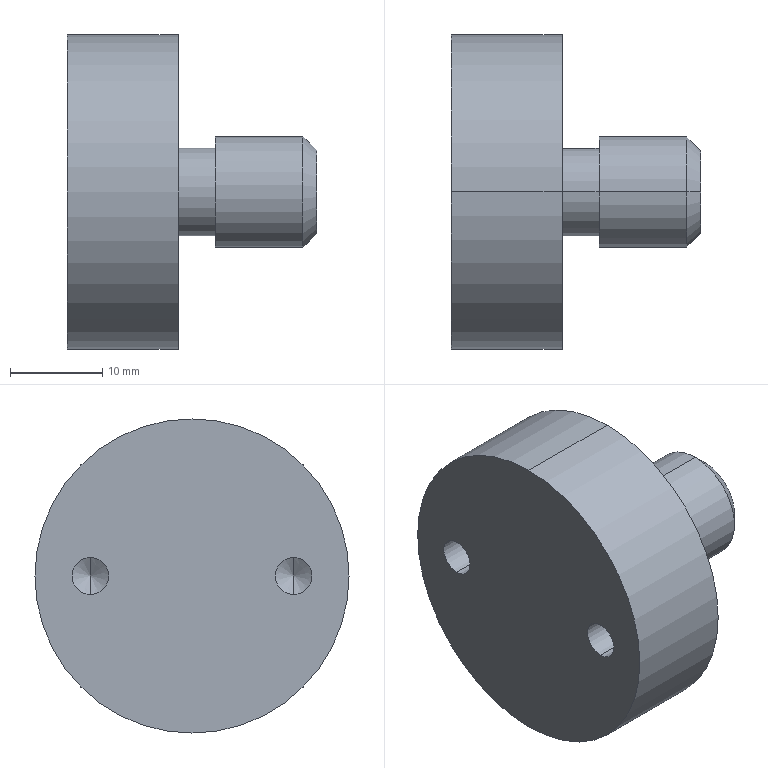Part | SolidWorks | features Chamfer 1, MirrorPattern 1, RevCut 1, Revolution 1 | 1 solid | 20 faces | box 27 x 34 x 34 mm | volume 12223 mm3 | cylinder 10 | cone 6 | plane 4 | commonest cylinder face diameters 4 x4 9.5 x2 12 x2 34 x2
STEP:
#1=CARTESIAN_POINT('',(6.,-11.,2.));
#2=VERTEX_POINT('',#1);
#3=CARTESIAN_POINT('',(6.,-11.,-2.));
#4=VERTEX_POINT('',#3);
#5=CARTESIAN_POINT('',(6.,-11.,0.));
#6=DIRECTION('',(1.,0.,0.));
#7=DIRECTION('',(0.,0.,1.));
#8=AXIS2_PLACEMENT_3D('',#5,#6,#7);
#9=CIRCLE('',#8,2.);
#10=EDGE_CURVE('',#2,#4,#9,.T.);
#11=ORIENTED_EDGE('',*,*,#10,.T.);
#12=CARTESIAN_POINT('',(0.,-11.,-2.));
#13=VERTEX_POINT('',#12);
#14=CARTESIAN_POINT('',(-2.467,-11.,-2.));
#15=DIRECTION('',(-1.,0.,0.));
#16=VECTOR('',#15,1000.);
#17=LINE('',#14,#16);
#18=EDGE_CURVE('',#4,#13,#17,.T.);
#19=ORIENTED_EDGE('',*,*,#18,.T.);
#20=CARTESIAN_POINT('',(0.,-11.,2.));
#21=VERTEX_POINT('',#20);
#22=CARTESIAN_POINT('',(0.,-11.,0.));
#23=DIRECTION('',(1.,0.,0.));
#24=DIRECTION('',(0.,0.,1.));
#25=AXIS2_PLACEMENT_3D('',#22,#23,#24);
#26=CIRCLE('',#25,2.);
#27=EDGE_CURVE('',#21,#13,#26,.T.);
#28=ORIENTED_EDGE('',*,*,#27,.F.);
#29=CARTESIAN_POINT('',(-2.467,-11.,2.));
#30=DIRECTION('',(-1.,0.,0.));
#31=VECTOR('',#30,1000.);
#32=LINE('',#29,#31);
#33=EDGE_CURVE('',#2,#21,#32,.T.);
#34=ORIENTED_EDGE('',*,*,#33,.F.);
#35=EDGE_LOOP('',(#11,#19,#28,#34));
#36=FACE_OUTER_BOUND('',#35,.T.);
#37=CARTESIAN_POINT('',(-2.467,-11.,0.));
#38=DIRECTION('',(-1.,0.,0.));
#39=DIRECTION('',(0.,0.,1.));
#40=AXIS2_PLACEMENT_3D('',#37,#38,#39);
#41=CYLINDRICAL_SURFACE('',#40,2.);
#42=ADVANCED_FACE('',(#36),#41,.F.);
#43=CARTESIAN_POINT('',(7.155,-11.,0.));
#44=VERTEX_POINT('',#43);
#45=CARTESIAN_POINT('',(7.155,-11.,0.));
#46=DIRECTION('',(-0.5,0.,0.866));
#47=VECTOR('',#46,1000.);
#48=LINE('',#45,#47);
#49=EDGE_CURVE('',#44,#2,#48,.T.);
#50=ORIENTED_EDGE('',*,*,#49,.F.);
#51=CARTESIAN_POINT('',(7.155,-11.,0.));
#52=DIRECTION('',(-0.5,0.,-0.866));
#53=VECTOR('',#52,1000.);
#54=LINE('',#51,#53);
#55=EDGE_CURVE('',#44,#4,#54,.T.);
#56=ORIENTED_EDGE('',*,*,#55,.T.);
#57=ORIENTED_EDGE('',*,*,#10,.F.);
#58=EDGE_LOOP('',(#50,#56,#57));
#59=FACE_OUTER_BOUND('',#58,.T.);
#60=CARTESIAN_POINT('',(-992.845,-11.,0.));
#61=DIRECTION('',(-1.,0.,0.));
#62=DIRECTION('',(0.,0.,1.));
#63=AXIS2_PLACEMENT_3D('',#60,#61,#62);
#64=CONICAL_SURFACE('',#63,1732.051,1.047);
#65=ADVANCED_FACE('',(#59),#64,.F.);
#66=CARTESIAN_POINT('',(6.,11.,-2.));
#67=VERTEX_POINT('',#66);
#68=CARTESIAN_POINT('',(6.,11.,2.));
#69=VERTEX_POINT('',#68);
#70=CARTESIAN_POINT('',(6.,11.,0.));
#71=DIRECTION('',(-1.,0.,0.));
#72=DIRECTION('',(0.,0.,1.));
#73=AXIS2_PLACEMENT_3D('',#70,#71,#72);
#74=CIRCLE('',#73,2.);
#75=EDGE_CURVE('',#67,#69,#74,.T.);
#76=ORIENTED_EDGE('',*,*,#75,.F.);
#77=CARTESIAN_POINT('',(0.,11.,-2.));
#78=VERTEX_POINT('',#77);
#79=CARTESIAN_POINT('',(-2.467,11.,-2.));
#80=DIRECTION('',(-1.,0.,0.));
#81=VECTOR('',#80,1000.);
#82=LINE('',#79,#81);
#83=EDGE_CURVE('',#67,#78,#82,.T.);
#84=ORIENTED_EDGE('',*,*,#83,.T.);
#85=CARTESIAN_POINT('',(0.,11.,2.));
#86=VERTEX_POINT('',#85);
#87=CARTESIAN_POINT('',(0.,11.,0.));
#88=DIRECTION('',(-1.,0.,0.));
#89=DIRECTION('',(0.,0.,1.));
#90=AXIS2_PLACEMENT_3D('',#87,#88,#89);
#91=CIRCLE('',#90,2.);
#92=EDGE_CURVE('',#78,#86,#91,.T.);
#93=ORIENTED_EDGE('',*,*,#92,.T.);
#94=CARTESIAN_POINT('',(-2.467,11.,2.));
#95=DIRECTION('',(-1.,0.,0.));
#96=VECTOR('',#95,1000.);
#97=LINE('',#94,#96);
#98=EDGE_CURVE('',#69,#86,#97,.T.);
#99=ORIENTED_EDGE('',*,*,#98,.F.);
#100=EDGE_LOOP('',(#76,#84,#93,#99));
#101=FACE_OUTER_BOUND('',#100,.T.);
#102=CARTESIAN_POINT('',(-2.467,11.,0.));
#103=DIRECTION('',(-1.,0.,0.));
#104=DIRECTION('',(0.,0.,1.));
#105=AXIS2_PLACEMENT_3D('',#102,#103,#104);
#106=CYLINDRICAL_SURFACE('',#105,2.);
#107=ADVANCED_FACE('',(#101),#106,.F.);
#108=CARTESIAN_POINT('',(7.155,11.,0.));
#109=VERTEX_POINT('',#108);
#110=CARTESIAN_POINT('',(7.155,11.,0.));
#111=DIRECTION('',(-0.5,0.,0.866));
#112=VECTOR('',#111,1000.);
#113=LINE('',#110,#112);
#114=EDGE_CURVE('',#109,#69,#113,.T.);
#115=ORIENTED_EDGE('',*,*,#114,.F.);
#116=CARTESIAN_POINT('',(7.155,11.,0.));
#117=DIRECTION('',(-0.5,0.,-0.866));
#118=VECTOR('',#117,1000.);
#119=LINE('',#116,#118);
#120=EDGE_CURVE('',#109,#67,#119,.T.);
#121=ORIENTED_EDGE('',*,*,#120,.T.);
#122=ORIENTED_EDGE('',*,*,#75,.T.);
#123=EDGE_LOOP('',(#115,#121,#122));
#124=FACE_OUTER_BOUND('',#123,.T.);
#125=CARTESIAN_POINT('',(-992.845,11.,0.));
#126=DIRECTION('',(-1.,0.,0.));
#127=DIRECTION('',(0.,0.,1.));
#128=AXIS2_PLACEMENT_3D('',#125,#126,#127);
#129=CONICAL_SURFACE('',#128,1732.051,1.047);
#130=ADVANCED_FACE('',(#124),#129,.F.);
#131=CARTESIAN_POINT('',(27.,0.,-4.5));
#132=VERTEX_POINT('',#131);
#133=CARTESIAN_POINT('',(27.,0.,4.5));
#134=VERTEX_POINT('',#133);
#135=CARTESIAN_POINT('',(27.,0.,0.));
#136=DIRECTION('',(1.,0.,0.));
#137=DIRECTION('',(0.,0.,1.));
#138=AXIS2_PLACEMENT_3D('',#135,#136,#137);
#139=CIRCLE('',#138,4.5);
#140=EDGE_CURVE('',#132,#134,#139,.T.);
#141=ORIENTED_EDGE('',*,*,#140,.F.);
#142=CARTESIAN_POINT('',(25.5,0.,-6.));
#143=VERTEX_POINT('',#142);
#144=CARTESIAN_POINT('',(25.5,0.,-6.));
#145=DIRECTION('',(-0.7071,0.,-0.7071));
#146=VECTOR('',#145,1000.);
#147=LINE('',#144,#146);
#148=EDGE_CURVE('',#132,#143,#147,.T.);
#149=ORIENTED_EDGE('',*,*,#148,.T.);
#150=CARTESIAN_POINT('',(25.5,0.,6.));
#151=VERTEX_POINT('',#150);
#152=CARTESIAN_POINT('',(25.5,0.,0.));
#153=DIRECTION('',(-1.,0.,0.));
#154=DIRECTION('',(0.,0.,1.));
#155=AXIS2_PLACEMENT_3D('',#152,#153,#154);
#156=CIRCLE('',#155,6.);
#157=EDGE_CURVE('',#151,#143,#156,.T.);
#158=ORIENTED_EDGE('',*,*,#157,.F.);
#159=CARTESIAN_POINT('',(25.5,0.,6.));
#160=DIRECTION('',(-0.7071,0.,0.7071));
#161=VECTOR('',#160,1000.);
#162=LINE('',#159,#161);
#163=EDGE_CURVE('',#134,#151,#162,.T.);
#164=ORIENTED_EDGE('',*,*,#163,.F.);
#165=EDGE_LOOP('',(#141,#149,#158,#164));
#166=FACE_OUTER_BOUND('',#165,.T.);
#167=CARTESIAN_POINT('',(25.5,0.,0.));
#168=DIRECTION('',(-1.,0.,0.));
#169=DIRECTION('',(0.,0.,1.));
#170=AXIS2_PLACEMENT_3D('',#167,#168,#169);
#171=CONICAL_SURFACE('',#170,6.,0.7854);
#172=ADVANCED_FACE('',(#166),#171,.T.);
#173=ORIENTED_EDGE('',*,*,#157,.T.);
#174=CARTESIAN_POINT('',(16.,0.,-6.));
#175=VERTEX_POINT('',#174);
#176=CARTESIAN_POINT('',(0.,0.,-6.));
#177=DIRECTION('',(-1.,0.,0.));
#178=VECTOR('',#177,1000.);
#179=LINE('',#176,#178);
#180=EDGE_CURVE('',#143,#175,#179,.T.);
#181=ORIENTED_EDGE('',*,*,#180,.T.);
#182=CARTESIAN_POINT('',(16.,0.,6.));
#183=VERTEX_POINT('',#182);
#184=CARTESIAN_POINT('',(16.,0.,0.));
#185=DIRECTION('',(-1.,0.,0.));
#186=DIRECTION('',(0.,0.,1.));
#187=AXIS2_PLACEMENT_3D('',#184,#185,#186);
#188=CIRCLE('',#187,6.);
#189=EDGE_CURVE('',#183,#175,#188,.T.);
#190=ORIENTED_EDGE('',*,*,#189,.F.);
#191=CARTESIAN_POINT('',(0.,0.,6.));
#192=DIRECTION('',(-1.,0.,0.));
#193=VECTOR('',#192,1000.);
#194=LINE('',#191,#193);
#195=EDGE_CURVE('',#151,#183,#194,.T.);
#196=ORIENTED_EDGE('',*,*,#195,.F.);
#197=EDGE_LOOP('',(#173,#181,#190,#196));
#198=FACE_OUTER_BOUND('',#197,.T.);
#199=CARTESIAN_POINT('',(0.,0.,0.));
#200=DIRECTION('',(-1.,0.,0.));
#201=DIRECTION('',(0.,0.,1.));
#202=AXIS2_PLACEMENT_3D('',#199,#200,#201);
#203=CYLINDRICAL_SURFACE('',#202,6.);
#204=ADVANCED_FACE('',(#198),#203,.T.);
#205=CARTESIAN_POINT('',(16.,0.,4.75));
#206=VERTEX_POINT('',#205);
#207=CARTESIAN_POINT('',(16.,0.,-4.75));
#208=VERTEX_POINT('',#207);
#209=CARTESIAN_POINT('',(16.,0.,0.));
#210=DIRECTION('',(-1.,0.,0.));
#211=DIRECTION('',(0.,0.,1.));
#212=AXIS2_PLACEMENT_3D('',#209,#210,#211);
#213=CIRCLE('',#212,4.75);
#214=EDGE_CURVE('',#206,#208,#213,.T.);
#215=ORIENTED_EDGE('',*,*,#214,.T.);
#216=CARTESIAN_POINT('',(12.,0.,-4.75));
#217=VERTEX_POINT('',#216);
#218=CARTESIAN_POINT('',(0.,0.,-4.75));
#219=DIRECTION('',(-1.,0.,0.));
#220=VECTOR('',#219,1000.);
#221=LINE('',#218,#220);
#222=EDGE_CURVE('',#208,#217,#221,.T.);
#223=ORIENTED_EDGE('',*,*,#222,.T.);
#224=CARTESIAN_POINT('',(12.,0.,4.75));
#225=VERTEX_POINT('',#224);
#226=CARTESIAN_POINT('',(12.,0.,0.));
#227=DIRECTION('',(-1.,0.,0.));
#228=DIRECTION('',(0.,0.,1.));
#229=AXIS2_PLACEMENT_3D('',#226,#227,#228);
#230=CIRCLE('',#229,4.75);
#231=EDGE_CURVE('',#225,#217,#230,.T.);
#232=ORIENTED_EDGE('',*,*,#231,.F.);
#233=CARTESIAN_POINT('',(0.,0.,4.75));
#234=DIRECTION('',(-1.,0.,0.));
#235=VECTOR('',#234,1000.);
#236=LINE('',#233,#235);
#237=EDGE_CURVE('',#206,#225,#236,.T.);
#238=ORIENTED_EDGE('',*,*,#237,.F.);
#239=EDGE_LOOP('',(#215,#223,#232,#238));
#240=FACE_OUTER_BOUND('',#239,.T.);
#241=CARTESIAN_POINT('',(0.,0.,0.));
#242=DIRECTION('',(-1.,0.,0.));
#243=DIRECTION('',(0.,0.,1.));
#244=AXIS2_PLACEMENT_3D('',#241,#242,#243);
#245=CYLINDRICAL_SURFACE('',#244,4.75);
#246=ADVANCED_FACE('',(#240),#245,.T.);
#247=CARTESIAN_POINT('',(12.,0.,17.));
#248=VERTEX_POINT('',#247);
#249=CARTESIAN_POINT('',(12.,0.,-17.));
#250=VERTEX_POINT('',#249);
#251=CARTESIAN_POINT('',(12.,0.,0.));
#252=DIRECTION('',(-1.,0.,0.));
#253=DIRECTION('',(0.,0.,1.));
#254=AXIS2_PLACEMENT_3D('',#251,#252,#253);
#255=CIRCLE('',#254,17.);
#256=EDGE_CURVE('',#248,#250,#255,.T.);
#257=ORIENTED_EDGE('',*,*,#256,.T.);
#258=CARTESIAN_POINT('',(0.,0.,-17.));
#259=VERTEX_POINT('',#258);
#260=CARTESIAN_POINT('',(0.,0.,-17.));
#261=DIRECTION('',(-1.,0.,0.));
#262=VECTOR('',#261,1000.);
#263=LINE('',#260,#262);
#264=EDGE_CURVE('',#250,#259,#263,.T.);
#265=ORIENTED_EDGE('',*,*,#264,.T.);
#266=CARTESIAN_POINT('',(0.,0.,17.));
#267=VERTEX_POINT('',#266);
#268=CARTESIAN_POINT('',(0.,0.,0.));
#269=DIRECTION('',(-1.,0.,0.));
#270=DIRECTION('',(0.,0.,1.));
#271=AXIS2_PLACEMENT_3D('',#268,#269,#270);
#272=CIRCLE('',#271,17.);
#273=EDGE_CURVE('',#267,#259,#272,.T.);
#274=ORIENTED_EDGE('',*,*,#273,.F.);
#275=CARTESIAN_POINT('',(0.,0.,17.));
#276=DIRECTION('',(-1.,0.,0.));
#277=VECTOR('',#276,1000.);
#278=LINE('',#275,#277);
#279=EDGE_CURVE('',#248,#267,#278,.T.);
#280=ORIENTED_EDGE('',*,*,#279,.F.);
#281=EDGE_LOOP('',(#257,#265,#274,#280));
#282=FACE_OUTER_BOUND('',#281,.T.);
#283=CARTESIAN_POINT('',(0.,0.,0.));
#284=DIRECTION('',(-1.,0.,0.));
#285=DIRECTION('',(0.,0.,1.));
#286=AXIS2_PLACEMENT_3D('',#283,#284,#285);
#287=CYLINDRICAL_SURFACE('',#286,17.);
#288=ADVANCED_FACE('',(#282),#287,.T.);
#289=ORIENTED_EDGE('',*,*,#27,.T.);
#290=CARTESIAN_POINT('',(0.,-11.,0.));
#291=DIRECTION('',(1.,0.,0.));
#292=DIRECTION('',(0.,0.,1.));
#293=AXIS2_PLACEMENT_3D('',#290,#291,#292);
#294=CIRCLE('',#293,2.);
#295=EDGE_CURVE('',#13,#21,#294,.T.);
#296=ORIENTED_EDGE('',*,*,#295,.T.);
#297=EDGE_LOOP('',(#289,#296));
#298=FACE_BOUND('',#297,.T.);
#299=CARTESIAN_POINT('',(0.,11.,0.));
#300=DIRECTION('',(-1.,0.,0.));
#301=DIRECTION('',(0.,0.,1.));
#302=AXIS2_PLACEMENT_3D('',#299,#300,#301);
#303=CIRCLE('',#302,2.);
#304=EDGE_CURVE('',#86,#78,#303,.T.);
#305=ORIENTED_EDGE('',*,*,#304,.F.);
#306=ORIENTED_EDGE('',*,*,#92,.F.);
#307=EDGE_LOOP('',(#305,#306));
#308=FACE_BOUND('',#307,.T.);
#309=ORIENTED_EDGE('',*,*,#273,.T.);
#310=CARTESIAN_POINT('',(0.,0.,0.));
#311=DIRECTION('',(-1.,0.,0.));
#312=DIRECTION('',(0.,0.,1.));
#313=AXIS2_PLACEMENT_3D('',#310,#311,#312);
#314=CIRCLE('',#313,17.);
#315=EDGE_CURVE('',#259,#267,#314,.T.);
#316=ORIENTED_EDGE('',*,*,#315,.T.);
#317=EDGE_LOOP('',(#309,#316));
#318=FACE_OUTER_BOUND('',#317,.T.);
#319=CARTESIAN_POINT('',(0.,0.,0.));
#320=DIRECTION('',(1.,0.,0.));
#321=DIRECTION('',(0.,0.,-1.));
#322=AXIS2_PLACEMENT_3D('',#319,#320,#321);
#323=PLANE('',#322);
#324=ADVANCED_FACE('',(#298,#308,#318),#323,.F.);
#325=ORIENTED_EDGE('',*,*,#264,.F.);
#326=CARTESIAN_POINT('',(12.,0.,0.));
#327=DIRECTION('',(-1.,0.,0.));
#328=DIRECTION('',(0.,0.,1.));
#329=AXIS2_PLACEMENT_3D('',#326,#327,#328);
#330=CIRCLE('',#329,17.);
#331=EDGE_CURVE('',#250,#248,#330,.T.);
#332=ORIENTED_EDGE('',*,*,#331,.T.);
#333=ORIENTED_EDGE('',*,*,#279,.T.);
#334=ORIENTED_EDGE('',*,*,#315,.F.);
#335=EDGE_LOOP('',(#325,#332,#333,#334));
#336=FACE_OUTER_BOUND('',#335,.T.);
#337=CARTESIAN_POINT('',(0.,0.,0.));
#338=DIRECTION('',(-1.,0.,0.));
#339=DIRECTION('',(0.,0.,1.));
#340=AXIS2_PLACEMENT_3D('',#337,#338,#339);
#341=CYLINDRICAL_SURFACE('',#340,17.);
#342=ADVANCED_FACE('',(#336),#341,.T.);
#343=ORIENTED_EDGE('',*,*,#256,.F.);
#344=ORIENTED_EDGE('',*,*,#331,.F.);
#345=EDGE_LOOP('',(#343,#344));
#346=FACE_OUTER_BOUND('',#345,.T.);
#347=ORIENTED_EDGE('',*,*,#231,.T.);
#348=CARTESIAN_POINT('',(12.,0.,0.));
#349=DIRECTION('',(-1.,0.,0.));
#350=DIRECTION('',(0.,0.,1.));
#351=AXIS2_PLACEMENT_3D('',#348,#349,#350);
#352=CIRCLE('',#351,4.75);
#353=EDGE_CURVE('',#217,#225,#352,.T.);
#354=ORIENTED_EDGE('',*,*,#353,.T.);
#355=EDGE_LOOP('',(#347,#354));
#356=FACE_BOUND('',#355,.T.);
#357=CARTESIAN_POINT('',(12.,17.,0.));
#358=DIRECTION('',(-1.,0.,0.));
#359=DIRECTION('',(0.,0.,1.));
#360=AXIS2_PLACEMENT_3D('',#357,#358,#359);
#361=PLANE('',#360);
#362=ADVANCED_FACE('',(#346,#356),#361,.F.);
#363=ORIENTED_EDGE('',*,*,#222,.F.);
#364=CARTESIAN_POINT('',(16.,0.,0.));
#365=DIRECTION('',(-1.,0.,0.));
#366=DIRECTION('',(0.,0.,1.));
#367=AXIS2_PLACEMENT_3D('',#364,#365,#366);
#368=CIRCLE('',#367,4.75);
#369=EDGE_CURVE('',#208,#206,#368,.T.);
#370=ORIENTED_EDGE('',*,*,#369,.T.);
#371=ORIENTED_EDGE('',*,*,#237,.T.);
#372=ORIENTED_EDGE('',*,*,#353,.F.);
#373=EDGE_LOOP('',(#363,#370,#371,#372));
#374=FACE_OUTER_BOUND('',#373,.T.);
#375=CARTESIAN_POINT('',(0.,0.,0.));
#376=DIRECTION('',(-1.,0.,0.));
#377=DIRECTION('',(0.,0.,1.));
#378=AXIS2_PLACEMENT_3D('',#375,#376,#377);
#379=CYLINDRICAL_SURFACE('',#378,4.75);
#380=ADVANCED_FACE('',(#374),#379,.T.);
#381=ORIENTED_EDGE('',*,*,#214,.F.);
#382=ORIENTED_EDGE('',*,*,#369,.F.);
#383=EDGE_LOOP('',(#381,#382));
#384=FACE_BOUND('',#383,.T.);
#385=ORIENTED_EDGE('',*,*,#189,.T.);
#386=CARTESIAN_POINT('',(16.,0.,0.));
#387=DIRECTION('',(-1.,0.,0.));
#388=DIRECTION('',(0.,0.,1.));
#389=AXIS2_PLACEMENT_3D('',#386,#387,#388);
#390=CIRCLE('',#389,6.);
#391=EDGE_CURVE('',#175,#183,#390,.T.);
#392=ORIENTED_EDGE('',*,*,#391,.T.);
#393=EDGE_LOOP('',(#385,#392));
#394=FACE_OUTER_BOUND('',#393,.T.);
#395=CARTESIAN_POINT('',(16.,4.75,0.));
#396=DIRECTION('',(1.,0.,0.));
#397=DIRECTION('',(0.,0.,-1.));
#398=AXIS2_PLACEMENT_3D('',#395,#396,#397);
#399=PLANE('',#398);
#400=ADVANCED_FACE('',(#384,#394),#399,.F.);
#401=ORIENTED_EDGE('',*,*,#180,.F.);
#402=CARTESIAN_POINT('',(25.5,0.,0.));
#403=DIRECTION('',(-1.,0.,0.));
#404=DIRECTION('',(0.,0.,1.));
#405=AXIS2_PLACEMENT_3D('',#402,#403,#404);
#406=CIRCLE('',#405,6.);
#407=EDGE_CURVE('',#143,#151,#406,.T.);
#408=ORIENTED_EDGE('',*,*,#407,.T.);
#409=ORIENTED_EDGE('',*,*,#195,.T.);
#410=ORIENTED_EDGE('',*,*,#391,.F.);
#411=EDGE_LOOP('',(#401,#408,#409,#410));
#412=FACE_OUTER_BOUND('',#411,.T.);
#413=CARTESIAN_POINT('',(0.,0.,0.));
#414=DIRECTION('',(-1.,0.,0.));
#415=DIRECTION('',(0.,0.,1.));
#416=AXIS2_PLACEMENT_3D('',#413,#414,#415);
#417=CYLINDRICAL_SURFACE('',#416,6.);
#418=ADVANCED_FACE('',(#412),#417,.T.);
#419=CARTESIAN_POINT('',(27.,0.,0.));
#420=DIRECTION('',(1.,0.,0.));
#421=DIRECTION('',(0.,0.,1.));
#422=AXIS2_PLACEMENT_3D('',#419,#420,#421);
#423=CIRCLE('',#422,4.5);
#424=EDGE_CURVE('',#134,#132,#423,.T.);
#425=ORIENTED_EDGE('',*,*,#424,.T.);
#426=ORIENTED_EDGE('',*,*,#140,.T.);
#427=EDGE_LOOP('',(#425,#426));
#428=FACE_OUTER_BOUND('',#427,.T.);
#429=CARTESIAN_POINT('',(27.,6.,0.));
#430=DIRECTION('',(-1.,0.,0.));
#431=DIRECTION('',(0.,0.,1.));
#432=AXIS2_PLACEMENT_3D('',#429,#430,#431);
#433=PLANE('',#432);
#434=ADVANCED_FACE('',(#428),#433,.F.);
#435=ORIENTED_EDGE('',*,*,#148,.F.);
#436=ORIENTED_EDGE('',*,*,#424,.F.);
#437=ORIENTED_EDGE('',*,*,#163,.T.);
#438=ORIENTED_EDGE('',*,*,#407,.F.);
#439=EDGE_LOOP('',(#435,#436,#437,#438));
#440=FACE_OUTER_BOUND('',#439,.T.);
#441=CARTESIAN_POINT('',(25.5,0.,0.));
#442=DIRECTION('',(-1.,0.,0.));
#443=DIRECTION('',(0.,0.,1.));
#444=AXIS2_PLACEMENT_3D('',#441,#442,#443);
#445=CONICAL_SURFACE('',#444,6.,0.7854);
#446=ADVANCED_FACE('',(#440),#445,.T.);
#447=ORIENTED_EDGE('',*,*,#120,.F.);
#448=ORIENTED_EDGE('',*,*,#114,.T.);
#449=CARTESIAN_POINT('',(6.,11.,0.));
#450=DIRECTION('',(-1.,0.,0.));
#451=DIRECTION('',(0.,0.,1.));
#452=AXIS2_PLACEMENT_3D('',#449,#450,#451);
#453=CIRCLE('',#452,2.);
#454=EDGE_CURVE('',#69,#67,#453,.T.);
#455=ORIENTED_EDGE('',*,*,#454,.T.);
#456=EDGE_LOOP('',(#447,#448,#455));
#457=FACE_OUTER_BOUND('',#456,.T.);
#458=CARTESIAN_POINT('',(-992.845,11.,0.));
#459=DIRECTION('',(-1.,0.,0.));
#460=DIRECTION('',(0.,0.,1.));
#461=AXIS2_PLACEMENT_3D('',#458,#459,#460);
#462=CONICAL_SURFACE('',#461,1732.051,1.047);
#463=ADVANCED_FACE('',(#457),#462,.F.);
#464=ORIENTED_EDGE('',*,*,#83,.F.);
#465=ORIENTED_EDGE('',*,*,#454,.F.);
#466=ORIENTED_EDGE('',*,*,#98,.T.);
#467=ORIENTED_EDGE('',*,*,#304,.T.);
#468=EDGE_LOOP('',(#464,#465,#466,#467));
#469=FACE_OUTER_BOUND('',#468,.T.);
#470=CARTESIAN_POINT('',(-2.467,11.,0.));
#471=DIRECTION('',(-1.,0.,0.));
#472=DIRECTION('',(0.,0.,1.));
#473=AXIS2_PLACEMENT_3D('',#470,#471,#472);
#474=CYLINDRICAL_SURFACE('',#473,2.);
#475=ADVANCED_FACE('',(#469),#474,.F.);
#476=ORIENTED_EDGE('',*,*,#55,.F.);
#477=ORIENTED_EDGE('',*,*,#49,.T.);
#478=CARTESIAN_POINT('',(6.,-11.,0.));
#479=DIRECTION('',(1.,0.,0.));
#480=DIRECTION('',(0.,0.,1.));
#481=AXIS2_PLACEMENT_3D('',#478,#479,#480);
#482=CIRCLE('',#481,2.);
#483=EDGE_CURVE('',#4,#2,#482,.T.);
#484=ORIENTED_EDGE('',*,*,#483,.F.);
#485=EDGE_LOOP('',(#476,#477,#484));
#486=FACE_OUTER_BOUND('',#485,.T.);
#487=CARTESIAN_POINT('',(-992.845,-11.,0.));
#488=DIRECTION('',(-1.,0.,0.));
#489=DIRECTION('',(0.,0.,1.));
#490=AXIS2_PLACEMENT_3D('',#487,#488,#489);
#491=CONICAL_SURFACE('',#490,1732.051,1.047);
#492=ADVANCED_FACE('',(#486),#491,.F.);
#493=ORIENTED_EDGE('',*,*,#18,.F.);
#494=ORIENTED_EDGE('',*,*,#483,.T.);
#495=ORIENTED_EDGE('',*,*,#33,.T.);
#496=ORIENTED_EDGE('',*,*,#295,.F.);
#497=EDGE_LOOP('',(#493,#494,#495,#496));
#498=FACE_OUTER_BOUND('',#497,.T.);
#499=CARTESIAN_POINT('',(-2.467,-11.,0.));
#500=DIRECTION('',(-1.,0.,0.));
#501=DIRECTION('',(0.,0.,1.));
#502=AXIS2_PLACEMENT_3D('',#499,#500,#501);
#503=CYLINDRICAL_SURFACE('',#502,2.);
#504=ADVANCED_FACE('',(#498),#503,.F.);
#505=CLOSED_SHELL('',(#42,#65,#107,#130,#172,#204,#246,#288,#324,#342,#362,#380,#400,#418,#434,#446,#463,#475,#492,#504));
#506=MANIFOLD_SOLID_BREP('',#505);
#507=CARTESIAN_POINT('',(0.,0.,0.));
#508=DIRECTION('',(0.,0.,1.));
#509=DIRECTION('',(1.,0.,0.));
#510=AXIS2_PLACEMENT_3D('',#507,#508,#509);
#511=(LENGTH_UNIT()NAMED_UNIT(*)SI_UNIT(.MILLI.,.METRE.));
#512=UNCERTAINTY_MEASURE_WITH_UNIT(LENGTH_MEASURE(0.00001),#511,'','');
#513=(NAMED_UNIT(*)PLANE_ANGLE_UNIT()SI_UNIT($,.RADIAN.));
#514=(NAMED_UNIT(*)SI_UNIT($,.STERADIAN.)SOLID_ANGLE_UNIT());
#515=(GEOMETRIC_REPRESENTATION_CONTEXT(3)GLOBAL_UNCERTAINTY_ASSIGNED_CONTEXT((#512))GLOBAL_UNIT_ASSIGNED_CONTEXT((#511,#513,#514))REPRESENTATION_CONTEXT('',''));
#516=ADVANCED_BREP_SHAPE_REPRESENTATION('',(#506,#510),#515);